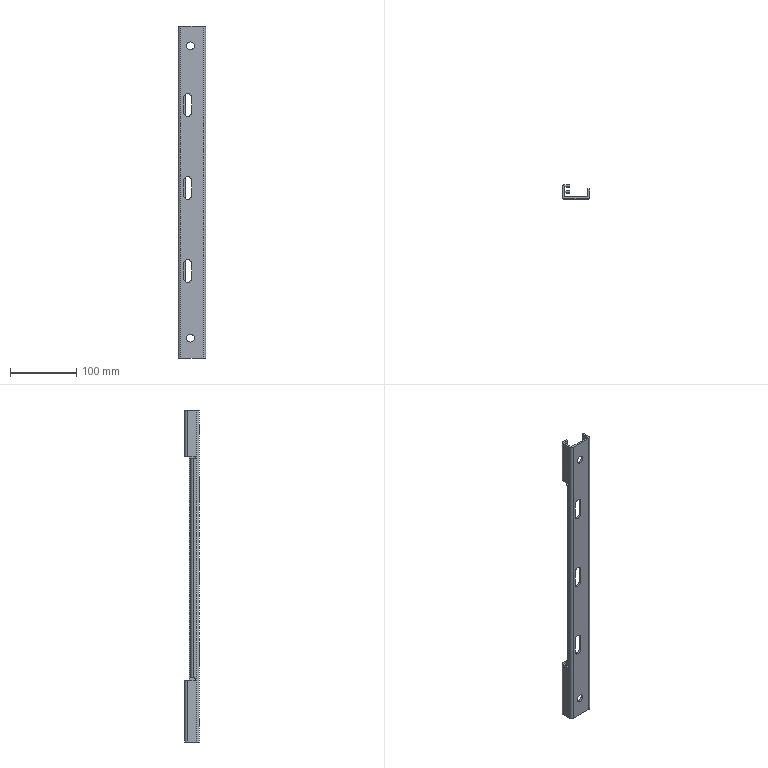Part | STEP file | 68377927 | 1 solid | 70 faces | box 41 x 21.5 x 500 mm | volume 101475 mm3 | plane 48 | cylinder 22 | commonest cylinder face diameters 12 x10 1.4 x5 7.4 x5 4 x2